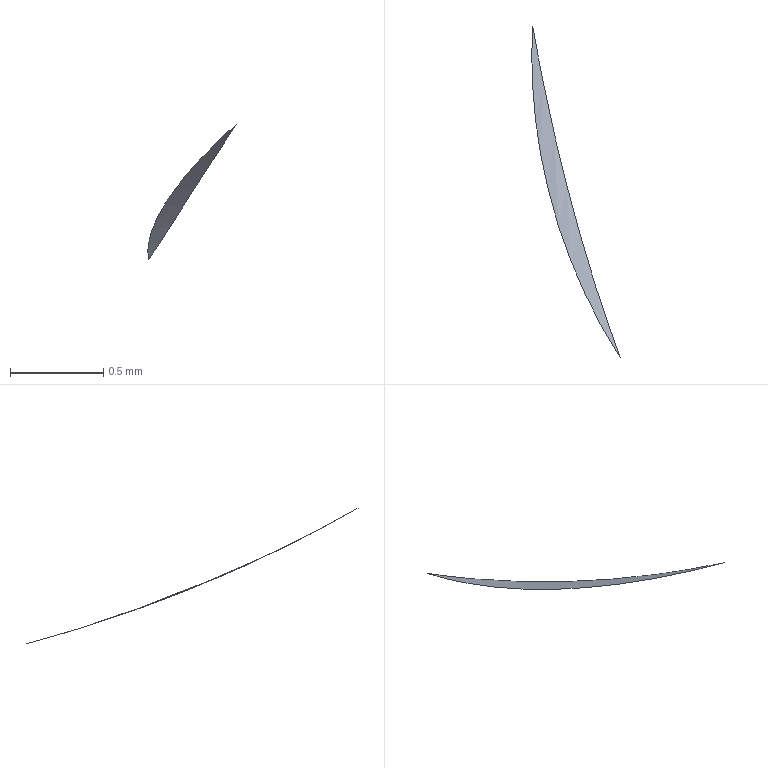Part | NX | features solid 2 | 1 solid | 2 faces | box 0.4748 x 1.783 x 0.7275 mm | volume 0.001212 mm3 | cylinder 1 | spline 1 | commonest cylinder face diameters 15 x1
STEP:
#1=CARTESIAN_POINT('',(584.077,138.895,-35.133));
#2=VERTEX_POINT('',#1);
#3=CARTESIAN_POINT('',(583.607,140.677,-35.86));
#4=VERTEX_POINT('',#3);
#5=CARTESIAN_POINT('',(583.608,140.677,-35.86));
#6=CARTESIAN_POINT('',(583.713,140.062,-35.698));
#7=CARTESIAN_POINT('',(583.869,139.461,-35.454));
#8=CARTESIAN_POINT('',(584.077,138.895,-35.133));
#9=B_SPLINE_CURVE_WITH_KNOTS('',3,(#5,#6,#7,#8),.UNSPECIFIED.,.F.,.F.,(4,4),(0.2444,0.4833),.UNSPECIFIED.);
#10=EDGE_CURVE('',#2,#4,#9,.F.);
#11=ORIENTED_EDGE('',*,*,#10,.F.);
#12=CARTESIAN_POINT('',(584.077,138.895,-35.133));
#13=CARTESIAN_POINT('',(583.753,139.403,-35.422));
#14=CARTESIAN_POINT('',(583.571,140.031,-35.689));
#15=CARTESIAN_POINT('',(583.607,140.677,-35.86));
#16=B_SPLINE_CURVE_WITH_KNOTS('',3,(#12,#13,#14,#15),.UNSPECIFIED.,.F.,.F.,(4,4),(-0.0001237,0.001883),.UNSPECIFIED.);
#17=EDGE_CURVE('',#4,#2,#16,.F.);
#18=ORIENTED_EDGE('',*,*,#17,.F.);
#19=EDGE_LOOP('',(#11,#18));
#20=FACE_BOUND('',#19,.T.);
#21=CARTESIAN_POINT('',(699.976,142.581,-28.61));
#22=DIRECTION('',(1.,-0.00013,0.000000201));
#23=DIRECTION('',(0.0001298,0.9979,0.0641));
#24=AXIS2_PLACEMENT_3D('',#21,#22,#23);
#25=CYLINDRICAL_SURFACE('',#24,7.5);
#26=ADVANCED_FACE('',(#20),#25,.T.);
#27=ORIENTED_EDGE('',*,*,#17,.T.);
#28=ORIENTED_EDGE('',*,*,#10,.T.);
#29=EDGE_LOOP('',(#27,#28));
#30=FACE_BOUND('',#29,.T.);
#31=CARTESIAN_POINT('',(584.081,138.885,-35.127));
#32=CARTESIAN_POINT('',(584.017,138.879,-35.124));
#33=CARTESIAN_POINT('',(583.953,138.874,-35.122));
#34=CARTESIAN_POINT('',(584.079,138.888,-35.129));
#35=CARTESIAN_POINT('',(584.016,138.883,-35.126));
#36=CARTESIAN_POINT('',(583.952,138.877,-35.123));
#37=CARTESIAN_POINT('',(584.078,138.891,-35.131));
#38=CARTESIAN_POINT('',(584.015,138.886,-35.128));
#39=CARTESIAN_POINT('',(583.951,138.88,-35.125));
#40=CARTESIAN_POINT('',(583.873,139.45,-35.448));
#41=CARTESIAN_POINT('',(583.81,139.445,-35.446));
#42=CARTESIAN_POINT('',(583.746,139.44,-35.444));
#43=CARTESIAN_POINT('',(583.713,140.056,-35.696));
#44=CARTESIAN_POINT('',(583.65,140.052,-35.695));
#45=CARTESIAN_POINT('',(583.586,140.048,-35.694));
#46=CARTESIAN_POINT('',(583.606,140.681,-35.861));
#47=CARTESIAN_POINT('',(583.543,140.678,-35.861));
#48=CARTESIAN_POINT('',(583.48,140.675,-35.86));
#49=CARTESIAN_POINT('',(583.605,140.685,-35.862));
#50=CARTESIAN_POINT('',(583.542,140.682,-35.862));
#51=CARTESIAN_POINT('',(583.479,140.679,-35.861));
#52=CARTESIAN_POINT('',(583.605,140.688,-35.863));
#53=CARTESIAN_POINT('',(583.542,140.685,-35.863));
#54=CARTESIAN_POINT('',(583.478,140.682,-35.862));
#55=(BOUNDED_SURFACE()B_SPLINE_SURFACE(3,2,((#31,#32,#33),(#34,#35,#36),(#37,#38,#39),(#40,#41,#42),(#43,#44,#45),(#46,#47,#48),(#49,#50,#51),(#52,#53,#54)),.UNSPECIFIED.,.F.,.F.,.F.)B_SPLINE_SURFACE_WITH_KNOTS((4,2,2,4),(3,3),(0.4985,0.5,0.75,0.7515),(0.,0.005649),.UNSPECIFIED.)GEOMETRIC_REPRESENTATION_ITEM()RATIONAL_B_SPLINE_SURFACE(((1.,0.9987,0.9973),(1.,0.9987,0.9973),(1.,0.9987,0.9973),(1.,0.9987,0.9974),(1.,0.9987,0.9974),(1.,0.9987,0.9974),(1.,0.9987,0.9974),(1.,0.9987,0.9974)))REPRESENTATION_ITEM('')SURFACE());
#56=ADVANCED_FACE('',(#30),#55,.T.);
#57=CLOSED_SHELL('',(#26,#56));
#58=MANIFOLD_SOLID_BREP('',#57);
#59=(LENGTH_UNIT()NAMED_UNIT(*)SI_UNIT(.MILLI.,.METRE.));
#60=UNCERTAINTY_MEASURE_WITH_UNIT(LENGTH_MEASURE(0.0508),#59,'','');
#61=(NAMED_UNIT(*)PLANE_ANGLE_UNIT()SI_UNIT($,.RADIAN.));
#62=(NAMED_UNIT(*)SI_UNIT($,.STERADIAN.)SOLID_ANGLE_UNIT());
#63=(GEOMETRIC_REPRESENTATION_CONTEXT(3)GLOBAL_UNCERTAINTY_ASSIGNED_CONTEXT((#60))GLOBAL_UNIT_ASSIGNED_CONTEXT((#59,#61,#62))REPRESENTATION_CONTEXT('',''));
#64=ADVANCED_BREP_SHAPE_REPRESENTATION('',(#58),#63);